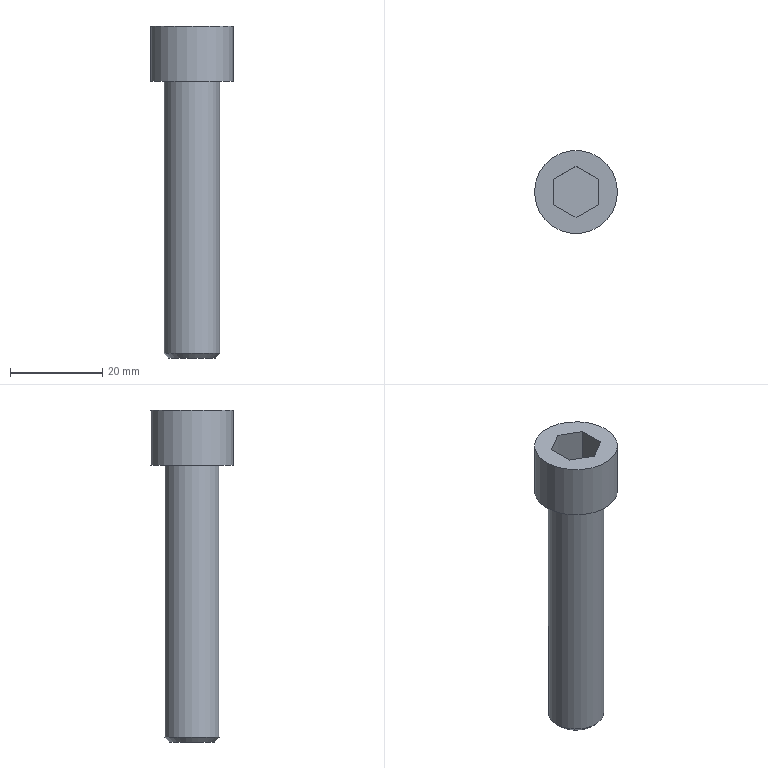Part | NX | features solid 2 | 1 solid | 13 faces | box 18 x 18 x 72 mm | volume 9247 mm3 | plane 10 | cylinder 2 | cone 1 | commonest cylinder face diameters 12 x1 18 x1
STEP:
#1=CARTESIAN_POINT('',(199.8,22.229,222.));
#2=VERTEX_POINT('',#1);
#3=CARTESIAN_POINT('',(195.,19.457,222.));
#4=VERTEX_POINT('',#3);
#5=CARTESIAN_POINT('',(197.4,20.843,222.));
#6=DIRECTION('',(-0.866,-0.5,0.));
#7=VECTOR('',#6,1000.);
#8=LINE('',#5,#7);
#9=EDGE_CURVE('',#2,#4,#8,.T.);
#10=ORIENTED_EDGE('',*,*,#9,.T.);
#11=CARTESIAN_POINT('',(190.2,22.229,222.));
#12=VERTEX_POINT('',#11);
#13=CARTESIAN_POINT('',(192.6,20.843,222.));
#14=DIRECTION('',(-0.866,0.5,0.));
#15=VECTOR('',#14,1000.);
#16=LINE('',#13,#15);
#17=EDGE_CURVE('',#4,#12,#16,.T.);
#18=ORIENTED_EDGE('',*,*,#17,.T.);
#19=CARTESIAN_POINT('',(190.2,27.771,222.));
#20=VERTEX_POINT('',#19);
#21=CARTESIAN_POINT('',(190.2,25.,222.));
#22=DIRECTION('',(0.,1.,0.));
#23=VECTOR('',#22,1000.);
#24=LINE('',#21,#23);
#25=EDGE_CURVE('',#12,#20,#24,.T.);
#26=ORIENTED_EDGE('',*,*,#25,.T.);
#27=CARTESIAN_POINT('',(195.,30.543,222.));
#28=VERTEX_POINT('',#27);
#29=CARTESIAN_POINT('',(192.6,29.157,222.));
#30=DIRECTION('',(0.866,0.5,0.));
#31=VECTOR('',#30,1000.);
#32=LINE('',#29,#31);
#33=EDGE_CURVE('',#20,#28,#32,.T.);
#34=ORIENTED_EDGE('',*,*,#33,.T.);
#35=CARTESIAN_POINT('',(199.8,27.771,222.));
#36=VERTEX_POINT('',#35);
#37=CARTESIAN_POINT('',(197.4,29.157,222.));
#38=DIRECTION('',(0.866,-0.5,0.));
#39=VECTOR('',#38,1000.);
#40=LINE('',#37,#39);
#41=EDGE_CURVE('',#28,#36,#40,.T.);
#42=ORIENTED_EDGE('',*,*,#41,.T.);
#43=CARTESIAN_POINT('',(199.8,25.,222.));
#44=DIRECTION('',(0.,-1.,0.));
#45=VECTOR('',#44,1000.);
#46=LINE('',#43,#45);
#47=EDGE_CURVE('',#36,#2,#46,.T.);
#48=ORIENTED_EDGE('',*,*,#47,.T.);
#49=EDGE_LOOP('',(#10,#18,#26,#34,#42,#48));
#50=FACE_BOUND('',#49,.T.);
#51=CARTESIAN_POINT('',(204.,25.,222.));
#52=VERTEX_POINT('',#51);
#53=CARTESIAN_POINT('',(195.,25.,222.));
#54=DIRECTION('',(0.,0.,1.));
#55=DIRECTION('',(1.,0.,0.));
#56=AXIS2_PLACEMENT_3D('',#53,#54,#55);
#57=CIRCLE('',#56,9.);
#58=EDGE_CURVE('',#52,#52,#57,.T.);
#59=ORIENTED_EDGE('',*,*,#58,.T.);
#60=EDGE_LOOP('',(#59));
#61=FACE_BOUND('',#60,.T.);
#62=CARTESIAN_POINT('',(195.,25.,222.));
#63=DIRECTION('',(0.,0.,1.));
#64=DIRECTION('',(-1.,0.,0.));
#65=AXIS2_PLACEMENT_3D('',#62,#63,#64);
#66=PLANE('',#65);
#67=ADVANCED_FACE('',(#50,#61),#66,.T.);
#68=CARTESIAN_POINT('',(201.,25.,210.));
#69=VERTEX_POINT('',#68);
#70=CARTESIAN_POINT('',(195.,25.,210.));
#71=DIRECTION('',(0.,0.,1.));
#72=DIRECTION('',(1.,0.,0.));
#73=AXIS2_PLACEMENT_3D('',#70,#71,#72);
#74=CIRCLE('',#73,6.);
#75=EDGE_CURVE('',#69,#69,#74,.T.);
#76=ORIENTED_EDGE('',*,*,#75,.T.);
#77=EDGE_LOOP('',(#76));
#78=FACE_BOUND('',#77,.T.);
#79=CARTESIAN_POINT('',(186.,25.,210.));
#80=VERTEX_POINT('',#79);
#81=CARTESIAN_POINT('',(195.,25.,210.));
#82=DIRECTION('',(0.,0.,-1.));
#83=DIRECTION('',(-1.,0.,0.));
#84=AXIS2_PLACEMENT_3D('',#81,#82,#83);
#85=CIRCLE('',#84,9.);
#86=EDGE_CURVE('',#80,#80,#85,.T.);
#87=ORIENTED_EDGE('',*,*,#86,.T.);
#88=EDGE_LOOP('',(#87));
#89=FACE_BOUND('',#88,.T.);
#90=CARTESIAN_POINT('',(195.,25.,210.));
#91=DIRECTION('',(0.,0.,-1.));
#92=DIRECTION('',(1.,0.,0.));
#93=AXIS2_PLACEMENT_3D('',#90,#91,#92);
#94=PLANE('',#93);
#95=ADVANCED_FACE('',(#78,#89),#94,.T.);
#96=ORIENTED_EDGE('',*,*,#58,.F.);
#97=EDGE_LOOP('',(#96));
#98=FACE_BOUND('',#97,.T.);
#99=ORIENTED_EDGE('',*,*,#86,.F.);
#100=EDGE_LOOP('',(#99));
#101=FACE_BOUND('',#100,.T.);
#102=CARTESIAN_POINT('',(195.,25.,210.));
#103=DIRECTION('',(0.,0.,1.));
#104=DIRECTION('',(-1.,0.,0.));
#105=AXIS2_PLACEMENT_3D('',#102,#103,#104);
#106=CYLINDRICAL_SURFACE('',#105,9.);
#107=ADVANCED_FACE('',(#98,#101),#106,.T.);
#108=ORIENTED_EDGE('',*,*,#9,.F.);
#109=CARTESIAN_POINT('',(199.8,22.229,214.8));
#110=VERTEX_POINT('',#109);
#111=CARTESIAN_POINT('',(199.8,22.229,214.8));
#112=DIRECTION('',(0.,0.,1.));
#113=VECTOR('',#112,1000.);
#114=LINE('',#111,#113);
#115=EDGE_CURVE('',#110,#2,#114,.T.);
#116=ORIENTED_EDGE('',*,*,#115,.F.);
#117=CARTESIAN_POINT('',(195.,19.457,214.8));
#118=VERTEX_POINT('',#117);
#119=CARTESIAN_POINT('',(199.8,22.229,214.8));
#120=DIRECTION('',(-0.866,-0.5,0.));
#121=VECTOR('',#120,1000.);
#122=LINE('',#119,#121);
#123=EDGE_CURVE('',#110,#118,#122,.T.);
#124=ORIENTED_EDGE('',*,*,#123,.T.);
#125=CARTESIAN_POINT('',(195.,19.457,214.8));
#126=DIRECTION('',(0.,0.,1.));
#127=VECTOR('',#126,1000.);
#128=LINE('',#125,#127);
#129=EDGE_CURVE('',#118,#4,#128,.T.);
#130=ORIENTED_EDGE('',*,*,#129,.T.);
#131=EDGE_LOOP('',(#108,#116,#124,#130));
#132=FACE_BOUND('',#131,.T.);
#133=CARTESIAN_POINT('',(197.4,20.843,220.8));
#134=DIRECTION('',(0.5,-0.866,0.));
#135=DIRECTION('',(0.866,0.5,0.));
#136=AXIS2_PLACEMENT_3D('',#133,#134,#135);
#137=PLANE('',#136);
#138=ADVANCED_FACE('',(#132),#137,.F.);
#139=ORIENTED_EDGE('',*,*,#47,.F.);
#140=CARTESIAN_POINT('',(199.8,27.771,214.8));
#141=VERTEX_POINT('',#140);
#142=CARTESIAN_POINT('',(199.8,27.771,214.8));
#143=DIRECTION('',(0.,0.,1.));
#144=VECTOR('',#143,1000.);
#145=LINE('',#142,#144);
#146=EDGE_CURVE('',#141,#36,#145,.T.);
#147=ORIENTED_EDGE('',*,*,#146,.F.);
#148=CARTESIAN_POINT('',(199.8,27.771,214.8));
#149=DIRECTION('',(0.,-1.,0.));
#150=VECTOR('',#149,1000.);
#151=LINE('',#148,#150);
#152=EDGE_CURVE('',#141,#110,#151,.T.);
#153=ORIENTED_EDGE('',*,*,#152,.T.);
#154=ORIENTED_EDGE('',*,*,#115,.T.);
#155=EDGE_LOOP('',(#139,#147,#153,#154));
#156=FACE_BOUND('',#155,.T.);
#157=CARTESIAN_POINT('',(199.8,25.,220.8));
#158=DIRECTION('',(1.,0.,0.));
#159=DIRECTION('',(0.,0.,1.));
#160=AXIS2_PLACEMENT_3D('',#157,#158,#159);
#161=PLANE('',#160);
#162=ADVANCED_FACE('',(#156),#161,.F.);
#163=ORIENTED_EDGE('',*,*,#41,.F.);
#164=CARTESIAN_POINT('',(195.,30.543,214.8));
#165=VERTEX_POINT('',#164);
#166=CARTESIAN_POINT('',(195.,30.543,214.8));
#167=DIRECTION('',(0.,0.,1.));
#168=VECTOR('',#167,1000.);
#169=LINE('',#166,#168);
#170=EDGE_CURVE('',#165,#28,#169,.T.);
#171=ORIENTED_EDGE('',*,*,#170,.F.);
#172=CARTESIAN_POINT('',(195.,30.543,214.8));
#173=DIRECTION('',(0.866,-0.5,0.));
#174=VECTOR('',#173,1000.);
#175=LINE('',#172,#174);
#176=EDGE_CURVE('',#165,#141,#175,.T.);
#177=ORIENTED_EDGE('',*,*,#176,.T.);
#178=ORIENTED_EDGE('',*,*,#146,.T.);
#179=EDGE_LOOP('',(#163,#171,#177,#178));
#180=FACE_BOUND('',#179,.T.);
#181=CARTESIAN_POINT('',(197.4,29.157,220.8));
#182=DIRECTION('',(0.5,0.866,0.));
#183=DIRECTION('',(-0.866,0.5,0.));
#184=AXIS2_PLACEMENT_3D('',#181,#182,#183);
#185=PLANE('',#184);
#186=ADVANCED_FACE('',(#180),#185,.F.);
#187=ORIENTED_EDGE('',*,*,#33,.F.);
#188=CARTESIAN_POINT('',(190.2,27.771,214.8));
#189=VERTEX_POINT('',#188);
#190=CARTESIAN_POINT('',(190.2,27.771,214.8));
#191=DIRECTION('',(0.,0.,1.));
#192=VECTOR('',#191,1000.);
#193=LINE('',#190,#192);
#194=EDGE_CURVE('',#189,#20,#193,.T.);
#195=ORIENTED_EDGE('',*,*,#194,.F.);
#196=CARTESIAN_POINT('',(190.2,27.771,214.8));
#197=DIRECTION('',(0.866,0.5,0.));
#198=VECTOR('',#197,1000.);
#199=LINE('',#196,#198);
#200=EDGE_CURVE('',#189,#165,#199,.T.);
#201=ORIENTED_EDGE('',*,*,#200,.T.);
#202=ORIENTED_EDGE('',*,*,#170,.T.);
#203=EDGE_LOOP('',(#187,#195,#201,#202));
#204=FACE_BOUND('',#203,.T.);
#205=CARTESIAN_POINT('',(192.6,29.157,220.8));
#206=DIRECTION('',(-0.5,0.866,0.));
#207=DIRECTION('',(-0.866,-0.5,0.));
#208=AXIS2_PLACEMENT_3D('',#205,#206,#207);
#209=PLANE('',#208);
#210=ADVANCED_FACE('',(#204),#209,.F.);
#211=ORIENTED_EDGE('',*,*,#25,.F.);
#212=CARTESIAN_POINT('',(190.2,22.229,214.8));
#213=VERTEX_POINT('',#212);
#214=CARTESIAN_POINT('',(190.2,22.229,214.8));
#215=DIRECTION('',(0.,0.,1.));
#216=VECTOR('',#215,1000.);
#217=LINE('',#214,#216);
#218=EDGE_CURVE('',#213,#12,#217,.T.);
#219=ORIENTED_EDGE('',*,*,#218,.F.);
#220=CARTESIAN_POINT('',(190.2,22.229,214.8));
#221=DIRECTION('',(0.,1.,0.));
#222=VECTOR('',#221,1000.);
#223=LINE('',#220,#222);
#224=EDGE_CURVE('',#213,#189,#223,.T.);
#225=ORIENTED_EDGE('',*,*,#224,.T.);
#226=ORIENTED_EDGE('',*,*,#194,.T.);
#227=EDGE_LOOP('',(#211,#219,#225,#226));
#228=FACE_BOUND('',#227,.T.);
#229=CARTESIAN_POINT('',(190.2,25.,220.8));
#230=DIRECTION('',(-1.,0.,0.));
#231=DIRECTION('',(0.,0.,-1.));
#232=AXIS2_PLACEMENT_3D('',#229,#230,#231);
#233=PLANE('',#232);
#234=ADVANCED_FACE('',(#228),#233,.F.);
#235=ORIENTED_EDGE('',*,*,#17,.F.);
#236=ORIENTED_EDGE('',*,*,#129,.F.);
#237=CARTESIAN_POINT('',(195.,19.457,214.8));
#238=DIRECTION('',(-0.866,0.5,0.));
#239=VECTOR('',#238,1000.);
#240=LINE('',#237,#239);
#241=EDGE_CURVE('',#118,#213,#240,.T.);
#242=ORIENTED_EDGE('',*,*,#241,.T.);
#243=ORIENTED_EDGE('',*,*,#218,.T.);
#244=EDGE_LOOP('',(#235,#236,#242,#243));
#245=FACE_BOUND('',#244,.T.);
#246=CARTESIAN_POINT('',(192.6,20.843,220.8));
#247=DIRECTION('',(-0.5,-0.866,0.));
#248=DIRECTION('',(0.866,-0.5,0.));
#249=AXIS2_PLACEMENT_3D('',#246,#247,#248);
#250=PLANE('',#249);
#251=ADVANCED_FACE('',(#245),#250,.F.);
#252=ORIENTED_EDGE('',*,*,#241,.F.);
#253=ORIENTED_EDGE('',*,*,#123,.F.);
#254=ORIENTED_EDGE('',*,*,#152,.F.);
#255=ORIENTED_EDGE('',*,*,#176,.F.);
#256=ORIENTED_EDGE('',*,*,#200,.F.);
#257=ORIENTED_EDGE('',*,*,#224,.F.);
#258=EDGE_LOOP('',(#252,#253,#254,#255,#256,#257));
#259=FACE_BOUND('',#258,.T.);
#260=CARTESIAN_POINT('',(195.,25.,214.8));
#261=DIRECTION('',(0.,0.,-1.));
#262=DIRECTION('',(1.,0.,0.));
#263=AXIS2_PLACEMENT_3D('',#260,#261,#262);
#264=PLANE('',#263);
#265=ADVANCED_FACE('',(#259),#264,.F.);
#266=CARTESIAN_POINT('',(190.,25.,150.));
#267=VERTEX_POINT('',#266);
#268=CARTESIAN_POINT('',(195.,25.,150.));
#269=DIRECTION('',(0.,0.,-1.));
#270=DIRECTION('',(-1.,0.,0.));
#271=AXIS2_PLACEMENT_3D('',#268,#269,#270);
#272=CIRCLE('',#271,5.);
#273=EDGE_CURVE('',#267,#267,#272,.T.);
#274=ORIENTED_EDGE('',*,*,#273,.T.);
#275=EDGE_LOOP('',(#274));
#276=FACE_BOUND('',#275,.T.);
#277=CARTESIAN_POINT('',(195.,25.,150.));
#278=DIRECTION('',(0.,0.,-1.));
#279=DIRECTION('',(-1.,0.,0.));
#280=AXIS2_PLACEMENT_3D('',#277,#278,#279);
#281=PLANE('',#280);
#282=ADVANCED_FACE('',(#276),#281,.T.);
#283=CARTESIAN_POINT('',(189.,25.,151.));
#284=VERTEX_POINT('',#283);
#285=CARTESIAN_POINT('',(195.,25.,151.));
#286=DIRECTION('',(0.,0.,-1.));
#287=DIRECTION('',(-1.,0.,0.));
#288=AXIS2_PLACEMENT_3D('',#285,#286,#287);
#289=CIRCLE('',#288,6.);
#290=EDGE_CURVE('',#284,#284,#289,.F.);
#291=ORIENTED_EDGE('',*,*,#290,.T.);
#292=EDGE_LOOP('',(#291));
#293=FACE_BOUND('',#292,.T.);
#294=ORIENTED_EDGE('',*,*,#75,.F.);
#295=EDGE_LOOP('',(#294));
#296=FACE_BOUND('',#295,.T.);
#297=CARTESIAN_POINT('',(195.,25.,210.));
#298=DIRECTION('',(0.,0.,-1.));
#299=DIRECTION('',(1.,0.,0.));
#300=AXIS2_PLACEMENT_3D('',#297,#298,#299);
#301=CYLINDRICAL_SURFACE('',#300,6.);
#302=ADVANCED_FACE('',(#293,#296),#301,.T.);
#303=ORIENTED_EDGE('',*,*,#290,.F.);
#304=EDGE_LOOP('',(#303));
#305=FACE_BOUND('',#304,.T.);
#306=ORIENTED_EDGE('',*,*,#273,.F.);
#307=EDGE_LOOP('',(#306));
#308=FACE_BOUND('',#307,.T.);
#309=CARTESIAN_POINT('',(195.,25.,150.));
#310=DIRECTION('',(0.,0.,1.));
#311=DIRECTION('',(1.,0.,0.));
#312=AXIS2_PLACEMENT_3D('',#309,#310,#311);
#313=CONICAL_SURFACE('',#312,5.,0.7854);
#314=ADVANCED_FACE('',(#305,#308),#313,.T.);
#315=CLOSED_SHELL('',(#67,#95,#107,#138,#162,#186,#210,#234,#251,#265,#282,#302,#314));
#316=MANIFOLD_SOLID_BREP('',#315);
#317=(LENGTH_UNIT()NAMED_UNIT(*)SI_UNIT(.MILLI.,.METRE.));
#318=UNCERTAINTY_MEASURE_WITH_UNIT(LENGTH_MEASURE(0.00001),#317,'','');
#319=(NAMED_UNIT(*)PLANE_ANGLE_UNIT()SI_UNIT($,.RADIAN.));
#320=(NAMED_UNIT(*)SI_UNIT($,.STERADIAN.)SOLID_ANGLE_UNIT());
#321=(GEOMETRIC_REPRESENTATION_CONTEXT(3)GLOBAL_UNCERTAINTY_ASSIGNED_CONTEXT((#318))GLOBAL_UNIT_ASSIGNED_CONTEXT((#317,#319,#320))REPRESENTATION_CONTEXT('',''));
#322=ADVANCED_BREP_SHAPE_REPRESENTATION('',(#316),#321);